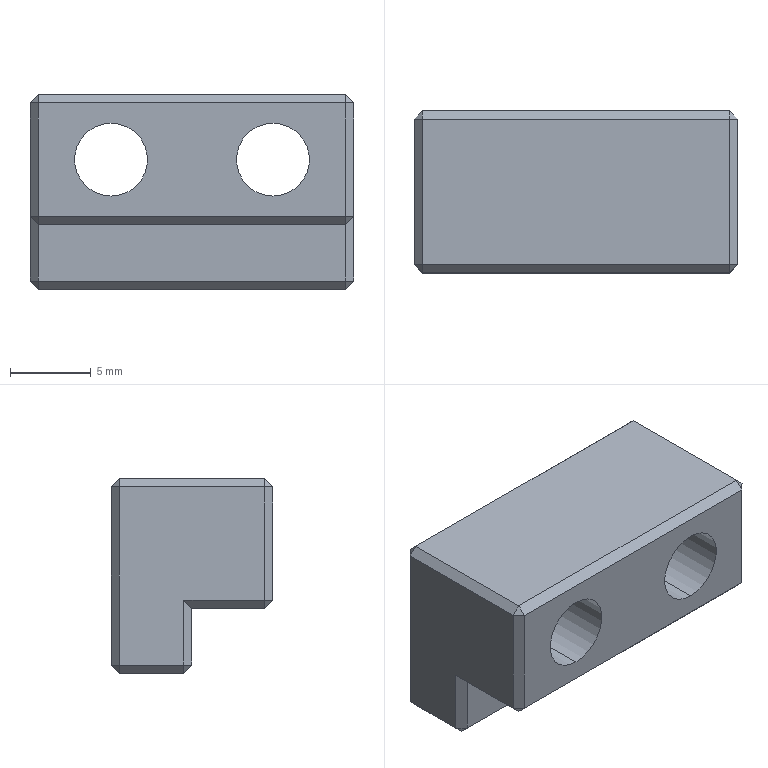Part | STEP file | 06-24 Cutter slide rail | 1 solid | 39 faces | box 20 x 10 x 12 mm | volume 1659 mm3 | plane 35 | cylinder 4 | commonest cylinder face diameters 4.5 x4